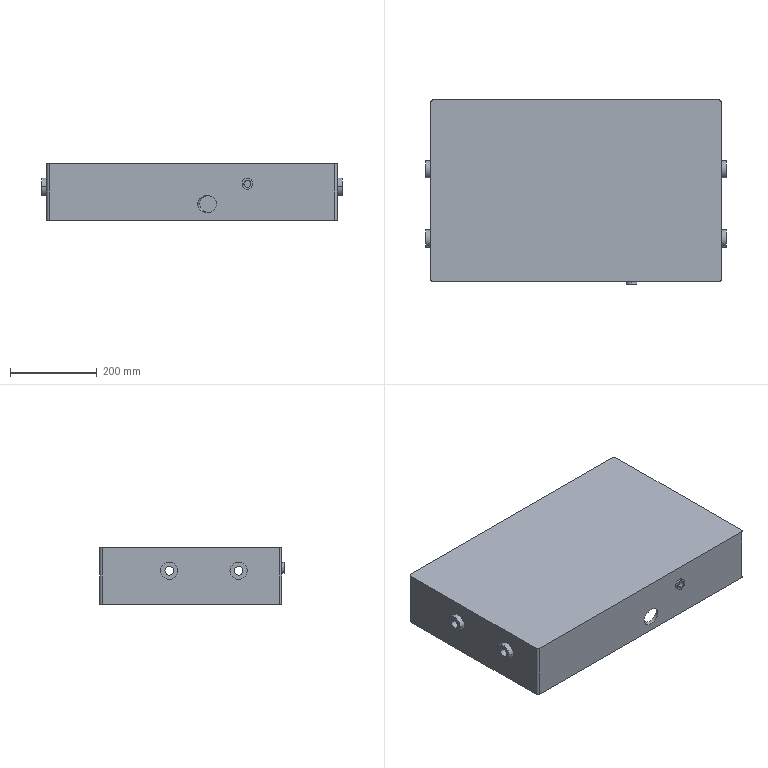Part | STEP file | PN_0006 Stainless steel water tank | 2 solids | 57 faces | box 694 x 425 x 130 mm | volume 5429065 mm3 | cylinder 36 | plane 21 | commonest cylinder face diameters 40 x18 20 x8 10 x4 25 x4 16 x2